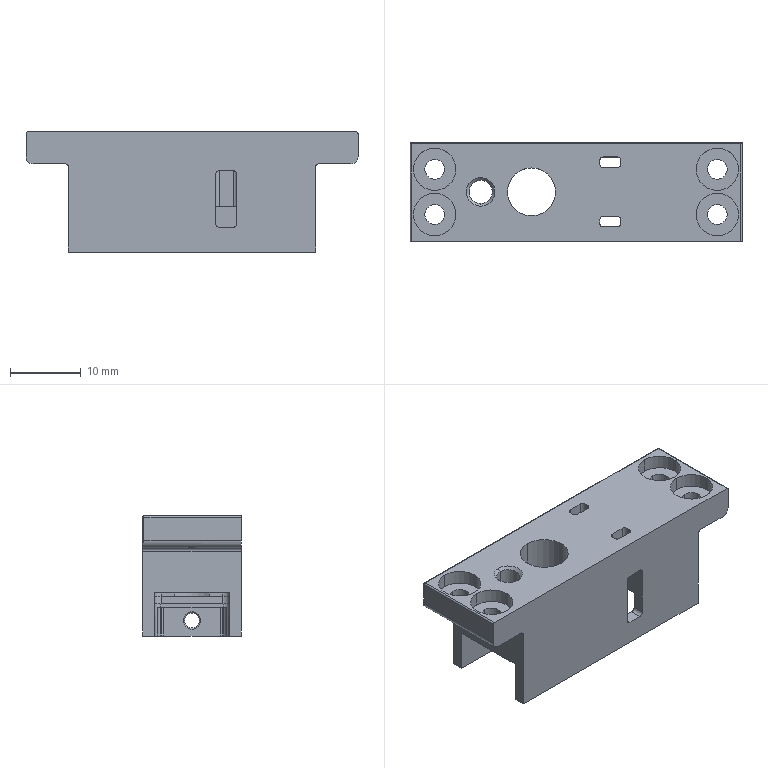NC program | NX | posted with a generic post | part box 47 x 14 x 17 mm
Lines 1496 to 2949 of 12912:
(CAVITY_MILL_COPY , TOOL : D4)
N2978 T10 M6
N2980 G54
N2982 G17 G0 G90 X8.1 Y-2.867 B0. C0. S9200 M3
N2984 G43 Z30. H10
N2986 Z0.627
N2988 G94 G1 Z-0.373 F1000.
N2990 G3 X8.887 Y-3.25 R1.
N2992 G1 X9.451 F1400.
N2994 G2 X10.016 Y-2.996 R2.
N2996 X11.2 Y-2.352 R2.14
N2998 G1 Y-1.338
N3000 G3 X10.8 Y-0.538 R1.
N3002 G1 Z0.627
N3004 G0 Z30.
N3006 X8.1 Y-2.867
N3008 Z0.255
N3010 G1 Z-0.745 F1000.
N3012 G3 X8.887 Y-3.25 R1.
N3014 G1 X9.451 F1400.
N3016 G2 X10.016 Y-2.996 R2.
N3018 X11.2 Y-2.352 R2.14
N3020 G1 Y-1.338
N3022 G3 X10.8 Y-0.538 R1.
N3024 G1 Z0.255
N3026 X8.1 Y-2.867 Z-0.118 F8000.
N3028 Z-1.118 F1000.
N3030 G3 X8.887 Y-3.25 R1.
N3032 G1 X9.451 F1400.
N3034 G2 X10.016 Y-2.996 R2.
N3036 X11.2 Y-2.352 R2.14
N3038 G1 Y-1.338
N3040 G3 X10.8 Y-0.538 R1.
N3042 G1 Z-0.118
N3044 X8.1 Y-2.867 Z-0.491 F8000.
N3046 Z-1.491 F1000.
N3048 G3 X8.887 Y-3.25 R1.
N3050 G1 X9.451 F1400.
N3052 G2 X10.016 Y-2.996 R2.
N3054 X11.2 Y-2.352 R2.14
N3056 G1 Y-1.338
N3058 G3 X10.8 Y-0.538 R1.
N3060 G1 Z-0.491
N3062 X8.1 Y-2.867 Z-0.864 F8000.
N3064 Z-1.864 F1000.
N3066 G3 X8.887 Y-3.25 R1.
N3068 G1 X9.451 F1400.
N3070 G2 X10.016 Y-2.996 R2.
N3072 X11.2 Y-2.352 R2.14
N3074 G1 Y-1.338
N3076 G3 X10.8 Y-0.538 R1.
N3078 G1 Z-0.864
N3080 X8.1 Y-2.867 Z-1.236 F8000.
N3082 Z-2.236 F1000.
N3084 G3 X8.887 Y-3.25 R1.
N3086 G1 X9.451 F1400.
N3088 G2 X10.016 Y-2.996 R2.
N3090 X11.2 Y-2.352 R2.14
N3092 G1 Y-1.338
N3094 G3 X10.8 Y-0.538 R1.
N3096 G1 Z-1.236
N3098 X8.1 Y-2.867 Z-1.609 F8000.
N3100 Z-2.609 F1000.
N3102 G3 X8.887 Y-3.25 R1.
N3104 G1 X9.451 F1400.
N3106 G2 X10.016 Y-2.996 R2.
N3108 X11.2 Y-2.352 R2.14
N3110 G1 Y-1.338
N3112 G3 X10.8 Y-0.538 R1.
N3114 G1 Z-1.609
N3116 X8.1 Y-2.867 Z-1.982 F8000.
N3118 Z-2.982 F1000.
N3120 G3 X8.887 Y-3.25 R1.
N3122 G1 X9.451 F1400.
N3124 G2 X10.016 Y-2.996 R2.
N3126 X11.2 Y-2.352 R2.14
N3128 G1 Y-1.338
N3130 G3 X10.8 Y-0.538 R1.
N3132 G1 Z-1.982
N3134 X8.1 Y-2.867 Z-2.355 F8000.
N3136 Z-3.355 F1000.
N3138 G3 X8.887 Y-3.25 R1.
N3140 G1 X9.451 F1400.
N3142 G2 X10.016 Y-2.996 R2.
N3144 X11.2 Y-2.352 R2.14
N3146 G1 Y-1.338
N3148 G3 X10.8 Y-0.538 R1.
N3150 G1 Z-2.355
N3152 X8.1 Y-2.867 Z-2.727 F8000.
N3154 Z-3.727 F1000.
N3156 G3 X8.887 Y-3.25 R1.
N3158 G1 X9.451 F1400.
N3160 G2 X10.016 Y-2.996 R2.
N3162 X11.2 Y-2.352 R2.14
N3164 G1 Y-1.338
N3166 G3 X10.8 Y-0.538 R1.
N3168 G1 Z-2.727
N3170 X8.1 Y-2.867 Z-3.1 F8000.
N3172 Z-4.1 F1000.
N3174 G3 X8.887 Y-3.25 R1.
N3176 G1 X9.451 F1400.
N3178 G2 X10.016 Y-2.996 R2.
N3180 X11.2 Y-2.352 R2.14
N3182 G1 Y-1.338
N3184 G3 X10.8 Y-0.538 R1.
N3186 G1 Z-3.1
N3188 X6.793 Y-2.95 Z-3.35 F8000.
N3190 Z-4.35 F1000.
N3192 G3 X7.593 Y-3.35 R1.
N3194 G1 X7.765 Y-3.349 F1400.
N3196 G2 X8.387 Y-3.25 R2.
N3198 G1 X8.7
N3200 Y-2.03
N3202 G3 X8.3 Y-1.23 R1.
N3204 G1 Z-3.35
N3206 X6.793 Y-2.95 Z-3.6 F8000.
N3208 Z-4.6 F1000.
N3210 G3 X7.593 Y-3.35 R1.
N3212 G1 X7.766 Y-3.349 F1400.
N3214 G2 X8.387 Y-3.25 R2.
N3216 G1 X8.7
N3218 Y-2.03
N3220 G3 X8.3 Y-1.23 R1.
N3222 G1 Z-3.6
N3224 X6.792 Y-2.95 Z-3.933 F8000.
N3226 Z-4.933 F1000.
N3228 G3 X7.592 Y-3.35 R1.
N3230 G1 X7.766 Y-3.349 F1400.
N3232 G2 X8.387 Y-3.25 R2.
N3234 G1 X8.7
N3236 Y-2.03
N3238 G3 X8.3 Y-1.23 R1.
N3240 G1 Z-3.933
N3242 X6.792 Y-2.95 Z-4.267 F8000.
N3244 Z-5.267 F1000.
N3246 G3 X7.592 Y-3.35 R1.
N3248 G1 X7.763 F1400.
N3250 X7.766 Y-3.349
N3252 G2 X8.387 Y-3.25 R2.
N3254 G1 X8.7
N3256 Y-2.03
N3258 G3 X8.3 Y-1.23 R1.
N3260 G1 Z-4.267
N3262 X6.791 Y-2.95 Z-4.6 F8000.
N3264 Z-5.6 F1000.
N3266 G3 X7.591 Y-3.35 R1.
N3268 G1 X7.763 F1400.
N3270 X7.767 Y-3.349
N3272 G2 X8.387 Y-3.25 R2.
N3274 G1 X8.7
N3276 Y-2.03
N3278 G3 X8.3 Y-1.23 R1.
N3280 G1 Z-4.6
N3282 X6.791 Y-2.95 Z-4.85 F8000.
N3284 Z-5.85 F1000.
N3286 G3 X7.591 Y-3.35 R1.
N3288 G1 X7.763 F1400.
N3290 X7.767 Y-3.349
N3292 G2 X8.387 Y-3.25 R2.
N3294 G1 X8.7
N3296 Y-2.029
N3298 G3 X8.3 Y-1.229 R1.
N3300 G1 Z-4.85
N3302 X6.791 Y-2.95 Z-5.1 F8000.
N3304 Z-6.1 F1000.
N3306 G3 X7.591 Y-3.35 R1.
N3308 G1 X7.763 F1400.
N3310 X7.767 Y-3.349
N3312 G2 X8.387 Y-3.25 R2.
N3314 G1 X8.7
N3316 Y-2.029
N3318 G3 X8.3 Y-1.229 R1.
N3320 G1 Z-5.1
N3322 X6.79 Y-2.95 Z-5.5 F8000.
N3324 Z-6.5 F1000.
N3326 G3 X7.59 Y-3.35 R1.
N3328 G1 X7.763 F1400.
N3330 X7.767 Y-3.349
N3332 G2 X8.387 Y-3.25 R2.
N3334 G1 X8.7
N3336 Y-2.029
N3338 G3 X8.3 Y-1.229 R1.
N3340 G1 Z-5.5
N3342 G0 Z30.
N3344 X10.8 Y0.538
N3346 Z0.627
N3348 G1 Z-0.373 F1000.
N3350 G3 X11.2 Y1.338 R1.
N3352 G1 Y2.352 F1400.
N3354 G2 X10.016 Y2.996 R2.14
N3356 X9.451 Y3.25 R2.
N3358 G1 X8.887
N3360 G3 X8.1 Y2.867 R1.
N3362 G1 Z0.627
N3364 G0 Z30.
N3366 X10.8 Y0.538
N3368 Z0.255
N3370 G1 Z-0.745 F1000.
N3372 G3 X11.2 Y1.338 R1.
N3374 G1 Y2.352 F1400.
N3376 G2 X10.016 Y2.996 R2.14
N3378 X9.451 Y3.25 R2.
N3380 G1 X8.887
N3382 G3 X8.1 Y2.867 R1.
N3384 G1 Z0.255
N3386 X10.8 Y0.538 Z-0.118 F8000.
N3388 Z-1.118 F1000.
N3390 G3 X11.2 Y1.338 R1.
N3392 G1 Y2.352 F1400.
N3394 G2 X10.016 Y2.996 R2.14
N3396 X9.451 Y3.25 R2.
N3398 G1 X8.887
N3400 G3 X8.1 Y2.867 R1.
N3402 G1 Z-0.118
N3404 X10.8 Y0.538 Z-0.491 F8000.
N3406 Z-1.491 F1000.
N3408 G3 X11.2 Y1.338 R1.
N3410 G1 Y2.352 F1400.
N3412 G2 X10.016 Y2.996 R2.14
N3414 X9.451 Y3.25 R2.
N3416 G1 X8.887
N3418 G3 X8.1 Y2.867 R1.
N3420 G1 Z-0.491
N3422 X10.8 Y0.538 Z-0.864 F8000.
N3424 Z-1.864 F1000.
N3426 G3 X11.2 Y1.338 R1.
N3428 G1 Y2.352 F1400.
N3430 G2 X10.016 Y2.996 R2.14
N3432 X9.451 Y3.25 R2.
N3434 G1 X8.887
N3436 G3 X8.1 Y2.867 R1.
N3438 G1 Z-0.864
N3440 X10.8 Y0.538 Z-1.236 F8000.
N3442 Z-2.236 F1000.
N3444 G3 X11.2 Y1.338 R1.
N3446 G1 Y2.352 F1400.
N3448 G2 X10.016 Y2.996 R2.14
N3450 X9.451 Y3.25 R2.
N3452 G1 X8.887
N3454 G3 X8.1 Y2.867 R1.
N3456 G1 Z-1.236
N3458 X10.8 Y0.538 Z-1.609 F8000.
N3460 Z-2.609 F1000.
N3462 G3 X11.2 Y1.338 R1.
N3464 G1 Y2.352 F1400.
N3466 G2 X10.016 Y2.996 R2.14
N3468 X9.451 Y3.25 R2.
N3470 G1 X8.887
N3472 G3 X8.1 Y2.867 R1.
N3474 G1 Z-1.609
N3476 X10.8 Y0.538 Z-1.982 F8000.
N3478 Z-2.982 F1000.
N3480 G3 X11.2 Y1.338 R1.
N3482 G1 Y2.352 F1400.
N3484 G2 X10.016 Y2.996 R2.14
N3486 X9.451 Y3.25 R2.
N3488 G1 X8.887
N3490 G3 X8.1 Y2.867 R1.
N3492 G1 Z-1.982
N3494 X10.8 Y0.538 Z-2.355 F8000.
N3496 Z-3.355 F1000.
N3498 G3 X11.2 Y1.338 R1.
N3500 G1 Y2.352 F1400.
N3502 G2 X10.016 Y2.996 R2.14
N3504 X9.451 Y3.25 R2.
N3506 G1 X8.887
N3508 G3 X8.1 Y2.867 R1.
N3510 G1 Z-2.355
N3512 X10.8 Y0.538 Z-2.727 F8000.
N3514 Z-3.727 F1000.
N3516 G3 X11.2 Y1.338 R1.
N3518 G1 Y2.352 F1400.
N3520 G2 X10.016 Y2.996 R2.14
N3522 X9.451 Y3.25 R2.
N3524 G1 X8.887
N3526 G3 X8.1 Y2.867 R1.
N3528 G1 Z-2.727
N3530 X10.8 Y0.538 Z-3.1 F8000.
N3532 Z-4.1 F1000.
N3534 G3 X11.2 Y1.338 R1.
N3536 G1 Y2.352 F1400.
N3538 G2 X10.016 Y2.996 R2.14
N3540 X9.451 Y3.25 R2.
N3542 G1 X8.887
N3544 G3 X8.1 Y2.867 R1.
N3546 G1 Z-3.1
N3548 X8.3 Y1.231 Z-3.35 F8000.
N3550 Z-4.35 F1000.
N3552 G3 X8.7 Y2.031 R1.
N3554 G1 Y3.25 F1400.
N3556 X8.387
N3558 G2 X7.763 Y3.35 R2.
N3560 G1 X7.596
N3562 G3 X6.796 Y2.95 R1.
N3564 G1 Z-3.35
N3566 X8.3 Y1.231 Z-3.6 F8000.
N3568 Z-4.6 F1000.
N3570 G3 X8.7 Y2.031 R1.
N3572 G1 Y3.25 F1400.
N3574 X8.387
N3576 G2 X7.763 Y3.35 R2.
N3578 G1 X7.596
N3580 G3 X6.796 Y2.95 R1.
N3582 G1 Z-3.6
N3584 X8.3 Y1.231 Z-3.933 F8000.
N3586 Z-4.933 F1000.
N3588 G3 X8.7 Y2.031 R1.
N3590 G1 Y3.25 F1400.
N3592 X8.387
N3594 G2 X7.763 Y3.35 R2.
N3596 G1 X7.596
N3598 G3 X6.796 Y2.95 R1.
N3600 G1 Z-3.933
N3602 X8.3 Y1.231 Z-4.267 F8000.
N3604 Z-5.267 F1000.
N3606 G3 X8.7 Y2.031 R1.
N3608 G1 Y3.25 F1400.
N3610 X8.387
N3612 G2 X7.763 Y3.35 R2.
N3614 G1 X7.596
N3616 G3 X6.796 Y2.95 R1.
N3618 G1 Z-4.267
N3620 X8.3 Y1.231 Z-4.6 F8000.
N3622 Z-5.6 F1000.
N3624 G3 X8.7 Y2.031 R1.
N3626 G1 Y3.25 F1400.
N3628 X8.387
N3630 G2 X7.763 Y3.35 R2.
N3632 G1 X7.596
N3634 G3 X6.796 Y2.95 R1.
N3636 G1 Z-4.6
N3638 X8.3 Y1.231 Z-4.85 F8000.
N3640 Z-5.85 F1000.
N3642 G3 X8.7 Y2.031 R1.
N3644 G1 Y3.25 F1400.
N3646 X8.387
N3648 G2 X7.763 Y3.35 R2.
N3650 G1 X7.596
N3652 G3 X6.796 Y2.95 R1.
N3654 G1 Z-4.85
N3656 X8.3 Y1.231 Z-5.1 F8000.
N3658 Z-6.1 F1000.
N3660 G3 X8.7 Y2.031 R1.
N3662 G1 Y3.25 F1400.
N3664 X8.387
N3666 G2 X7.763 Y3.35 R2.
N3668 G1 X7.596
N3670 G3 X6.796 Y2.95 R1.
N3672 G1 Z-5.1
N3674 X8.3 Y1.231 Z-5.5 F8000.
N3676 Z-6.5 F1000.
N3678 G3 X8.7 Y2.031 R1.
N3680 G1 Y3.25 F1400.
N3682 X8.387
N3684 G2 X7.763 Y3.35 R2.
N3686 G1 X7.596
N3688 G3 X6.796 Y2.95 R1.
N3690 G1 Z-5.5
N3692 G0 Z30.
N3694 X3.699
N3696 Z-3.933
N3698 G1 Z-4.933 F1000.
N3700 G3 X2.899 Y3.35 R1.
N3702 G1 X1.6 F1400.
N3704 Y2.051
N3706 G3 X2. Y1.251 R1.
N3708 G1 Z-3.933
N3710 X3.699 Y2.95 Z-4.267 F8000.
N3712 Z-5.267 F1000.
N3714 G3 X2.899 Y3.35 R1.
N3716 G1 X1.6 F1400.
N3718 Y2.051
N3720 G3 X2. Y1.251 R1.
N3722 G1 Z-4.267
N3724 X3.699 Y2.95 Z-4.6 F8000.
N3726 Z-5.6 F1000.
N3728 G3 X2.899 Y3.35 R1.
N3730 G1 X1.6 F1400.
N3732 Y2.051
N3734 G3 X2. Y1.251 R1.
N3736 G1 Z-4.6
N3738 X3.699 Y2.95 Z-4.85 F8000.
N3740 Z-5.85 F1000.
N3742 G3 X2.899 Y3.35 R1.
N3744 G1 X1.6 F1400.
N3746 Y2.051
N3748 G3 X2. Y1.251 R1.
N3750 G1 Z-4.85
N3752 X3.699 Y2.95 Z-5.1 F8000.
N3754 Z-6.1 F1000.
N3756 G3 X2.899 Y3.35 R1.
N3758 G1 X1.6 F1400.
N3760 Y2.051
N3762 G3 X2. Y1.251 R1.
N3764 G1 Z-5.1
N3766 X3.699 Y2.95 Z-5.5 F8000.
N3768 Z-6.5 F1000.
N3770 G3 X2.899 Y3.35 R1.
N3772 G1 X1.6 F1400.
N3774 Y2.051
N3776 G3 X2. Y1.251 R1.
N3778 G1 Z-5.5
N3780 G0 Z30.
N3782 Y-1.251
N3784 Z-3.933
N3786 G1 Z-4.933 F1000.
N3788 G3 X1.6 Y-2.051 R1.
N3790 G1 Y-3.35 F1400.
N3792 X2.899
N3794 G3 X3.699 Y-2.95 R1.
N3796 G1 Z-3.933
N3798 X2. Y-1.251 Z-4.267 F8000.
N3800 Z-5.267 F1000.
N3802 G3 X1.6 Y-2.051 R1.
N3804 G1 Y-3.35 F1400.
N3806 X2.899
N3808 G3 X3.699 Y-2.95 R1.
N3810 G1 Z-4.267
N3812 X2. Y-1.251 Z-4.6 F8000.
N3814 Z-5.6 F1000.
N3816 G3 X1.6 Y-2.051 R1.
N3818 G1 Y-3.35 F1400.
N3820 X2.899
N3822 G3 X3.699 Y-2.95 R1.
N3824 G1 Z-4.6
N3826 X2. Y-1.251 Z-4.85 F8000.
N3828 Z-5.85 F1000.
N3830 G3 X1.6 Y-2.051 R1.
N3832 G1 Y-3.35 F1400.
N3834 X2.899
N3836 G3 X3.699 Y-2.95 R1.
N3838 G1 Z-4.85
N3840 X2. Y-1.251 Z-5.1 F8000.
N3842 Z-6.1 F1000.
N3844 G3 X1.6 Y-2.051 R1.
N3846 G1 Y-3.35 F1400.
N3848 X2.899
N3850 G3 X3.699 Y-2.95 R1.
N3852 G1 Z-5.1
N3854 X2. Y-1.251 Z-5.5 F8000.
N3856 Z-6.5 F1000.
N3858 G3 X1.6 Y-2.051 R1.
N3860 G1 Y-3.35 F1400.
N3862 X2.899
N3864 G3 X3.699 Y-2.95 R1.
N3866 G1 Z-5.5
N3868 G0 Z30.
N3870 X-6.099
N3872 Z-3.933
N3874 G1 Z-4.933 F1000.
N3876 G3 X-5.299 Y-3.35 R1.
N3878 G1 X-4. F1400.
N3880 Y-2.051
N3882 G3 X-4.4 Y-1.251 R1.
N3884 G1 Z-3.933
N3886 X-6.099 Y-2.95 Z-4.267 F8000.
N3888 Z-5.267 F1000.
N3890 G3 X-5.299 Y-3.35 R1.
N3892 G1 X-4. F1400.
N3894 Y-2.051
N3896 G3 X-4.4 Y-1.251 R1.
N3898 G1 Z-4.267
N3900 X-6.099 Y-2.95 Z-4.6 F8000.
N3902 Z-5.6 F1000.
N3904 G3 X-5.299 Y-3.35 R1.
N3906 G1 X-4. F1400.
N3908 Y-2.051
N3910 G3 X-4.4 Y-1.251 R1.
N3912 G1 Z-4.6
N3914 X-7.098 Y-2.95 Z-4.85 F8000.
N3916 Z-5.85 F1000.
N3918 G3 X-6.298 Y-3.35 R1.
N3920 G1 X-5. F1400.
N3922 Y-2.433
N3924 G2 X-4.964 Y-2.058 R2.
N3926 G3 X-5.12 Y-1.308 R1.
N3928 G1 Z-4.85
N3930 X-7.098 Y-2.95 Z-5.1 F8000.
N3932 Z-6.1 F1000.
N3934 G3 X-6.298 Y-3.35 R1.
N3936 G1 X-5. F1400.
N3938 Y-2.433
N3940 G2 X-4.964 Y-2.058 R2.
N3942 G3 X-5.12 Y-1.308 R1.
N3944 G1 Z-5.1
N3946 G0 Z30.
N3948 X-4.4 Y1.251
N3950 Z-3.933
N3952 G1 Z-4.933 F1000.
N3954 G3 X-4. Y2.051 R1.
N3956 G1 Y3.35 F1400.
N3958 X-5.299
N3960 G3 X-6.099 Y2.95 R1.
N3962 G1 Z-3.933
N3964 X-4.4 Y1.251 Z-4.267 F8000.
N3966 Z-5.267 F1000.
N3968 G3 X-4. Y2.051 R1.
N3970 G1 Y3.35 F1400.
N3972 X-5.299
N3974 G3 X-6.099 Y2.95 R1.
N3976 G1 Z-4.267
N3978 X-4.4 Y1.251 Z-4.6 F8000.
N3980 Z-5.6 F1000.
N3982 G3 X-4. Y2.051 R1.
N3984 G1 Y3.35 F1400.
N3986 X-5.299
N3988 G3 X-6.099 Y2.95 R1.
N3990 G1 Z-4.6
N3992 X-5.12 Y1.308 Z-4.85 F8000.
N3994 Z-5.85 F1000.
N3996 G3 X-4.964 Y2.058 R1.
N3998 G2 X-5. Y2.433 R2. F1400.
N4000 G1 Y3.35
N4002 X-6.298
N4004 G3 X-7.098 Y2.95 R1.
N4006 G1 Z-4.85
N4008 X-5.12 Y1.308 Z-5.1 F8000.
N4010 Z-6.1 F1000.
N4012 G3 X-4.964 Y2.058 R1.
N4014 G2 X-5. Y2.433 R2. F1400.
N4016 G1 Y3.35
N4018 X-6.298
N4020 G3 X-7.098 Y2.95 R1.
N4022 G1 Z-5.1
N4024 G0 Z30.
(FLOOR_WALL_COPY_COPY , TOOL : D4)
N4026 X25.808 Y9.734 S9500
N4028 Z-11.
N4030 G1 Z-12.5 F1000.
N4032 X24.996 Y9.591
N4034 G3 X24.5 Y9. R0.6
N4036 G1 Y-9.
N4038 X20.2
N4040 Y9.
N4042 X24.5
N4044 X22.7 Y7.2
N4046 Y-7.2
N4048 X22.
N4050 Y7.2
N4052 X22.7
N4054 G3 X23.291 Y7.696 R0.6
N4056 G1 X23.785 Y10.5
N4058 Z-11.
N4060 G0 Z30.
N4062 X20.496
N4064 Z-11.
N4066 G1 Z-12.5
N4068 Y9.591
N4070 G3 X20. Y9. R0.6
N4072 G1 Y-9.
N4074 G3 X20.496 Y-9.591 R0.6
N4076 G1 Y-10.5
N4078 Z-11.
N4080 G0 Z30.
N4082 X7.2 Y-1.85
N4084 Z-2.6
N4086 G1 Z-4.1
N4088 X9.196 Y-2.459
N4090 G3 X8.7 Y-3.05 R0.6
N4092 G1 Y3.05
N4094 X9.393
N4096 G3 X9.909 Y2.818 R2.2
N4098 X11. Y2.191 R2.34
N4100 G1 Y-2.191
N4102 G3 X9.909 Y-2.818 R2.34
N4104 X9.393 Y-3.05 R2.2
N4106 G1 X8.7
N4108 G3 X9.291 Y-2.554 R0.6
N4110 G1 X7.2 Y-1.85
N4112 Z-2.6
N4114 G0 Z30.
N4116 Z-2.6
N4118 G1 Z-4.1
N4120 X8.109 Y-2.754
N4122 G3 X8.7 Y-3.25 R0.6
N4124 G1 X9.451
N4126 G2 X10.016 Y-2.996 R2.
N4128 X11.2 Y-2.352 R2.14
N4130 G1 Y2.352
N4132 G2 X10.016 Y2.996 R2.14
N4134 X9.451 Y3.25 R2.
N4136 G1 X8.7
N4138 G3 X8.109 Y2.754 R0.6
N4140 G1 X7.2 Y1.85
N4142 Z-2.6
N4144 G0 Z30.
N4146 X7.141 Y-2.654
N4148 Z-5.
N4150 G1 Z-6.5
N4152 G3 X7.732 Y-3.15 R0.6
N4154 G1 X1.8
N4156 Y3.15
N4158 X7.732
N4160 G3 X8.387 Y3.05 R2.2
N4162 G1 X8.5
N4164 Y-3.05
N4166 X8.387
N4168 G3 X7.732 Y-3.15 R2.2
N4170 G1 X6.1 Y-0.75
N4172 X4.2
N4174 Y0.75
N4176 X6.1
N4178 Y-0.75
N4180 X8.204 Y-1.341
N4182 G3 X8.7 Y-0.75 R0.6
N4184 G1 Y3.25
N4186 X8.387
N4188 G2 X7.763 Y3.35 R2.
N4190 G1 X1.6
N4192 Y-3.35
N4194 X7.763
N4196 G2 X8.387 Y-3.25 R2.
N4198 G1 X8.7
N4200 Y-0.75
N4202 G3 X8.204 Y-0.159 R0.6
N4204 G1 X7.2 Y0.018
N4206 Z-5.
N4208 G0 Z30.
N4210 X3.1 Y1.85
N4212 Z-3.1
N4214 G1 Z-4.6
N4216 X1.104 Y2.559
N4218 G3 X1.6 Y3.15 R0.6
N4220 G1 Y-3.15
N4222 X-4.
N4224 Y3.15
N4226 X1.6
N4228 X-0.8 Y0.75
N4230 Y-0.75
N4232 X-1.6
N4234 Y0.75
N4236 X-0.8
N4238 G3 X-0.209 Y1.246 R0.6
N4240 G1 X3.1
N4242 Z-3.1
N4244 G0 Z30.
N4246 Y1.85
N4248 Z-3.1
N4250 G1 Z-4.6
N4252 X2.191 Y2.854
N4254 G3 X1.6 Y3.35 R0.6
N4256 G1 X-4.
N4258 G3 X-4.591 Y2.854 R0.6
N4260 G1 X-5.5 Y1.85
N4262 Z-3.1
N4264 G0 Z30.
N4266 Y-1.85
N4268 Z-3.1
N4270 G1 Z-4.6
N4272 X-4.591 Y-2.854
N4274 G3 X-4. Y-3.35 R0.6
N4276 G1 X1.59
N4278 G3 X2.181 Y-2.854 R0.6
N4280 G1 X3.1 Y-1.85
N4282 Z-3.1
N4284 G0 Z30.
N4286 X-5.733
N4288 Z-4.1
N4290 G1 Z-5.6
N4292 X-5.591 Y-2.654
N4294 G3 X-5. Y-3.15 R0.6
N4296 G1 X-4.2
N4298 Y3.15
N4300 X-5.
N4302 G3 X-5.615 Y2.685 R0.6
N4304 G1 X-5.806 Y1.85
N4306 Z-4.1
N4308 G0 Z30.
N4310 X-5.99 Y-0.591
N4312 Z-4.1
N4314 G1 Z-5.6
N4316 X-5.591 Y-2.854
N4318 G3 X-5. Y-3.35 R0.6
N4320 G1 X-4.
N4322 Y3.35
N4324 X-4.99
N4326 G3 X-5.581 Y2.854 R0.6
N4328 G1 X-5.982 Y0.58
N4330 Z-4.1
N4332 G0 Z30.
N4334 X-6.052 Y0.546
N4336 Z-4.6
N4338 G1 Z-6.1
N4340 X-5.322 Y2.155
N4342 G3 X-5.2 Y1.789 R0.3
N4344 X-5.2 Y-1.789 R-2.1
N4346 G1 Y-3.15
N4348 X-19.5
N4350 Y3.15
N4352 X-5.2
N4354 Y1.789
N4356 G3 X-7.974 Y1.268 R2.1
N4358 G1 X-10.737 Y0.75
N4360 G3 X-10.737 Y-0.75 R4.5
N4362 G1 X-17.1
N4364 Y0.75
N4366 X-10.737
N4368 G3 X-10.146 Y1.246 R0.6
N4370 G1 X-6.871 Y0.185
N4372 Z-4.6
N4374 G0 Z30.
N4376 X-5.747 Y0.233
N4378 Z-4.6
N4380 G1 Z-6.1
N4382 X-4.78 Y0.642
N4384 G3 X-4.732 Y1.411 R0.6
N4386 G1 X-5. Y1.776
N4388 Y3.35
N4390 X-19.5
N4392 G3 X-20.091 Y2.854 R0.6
N4394 G1 X-21.
N4396 Z-4.6
N4398 G0 Z30.
N4400 Y-2.854
N4402 Z-4.6
N4404 G1 Z-6.1
N4406 X-20.091
N4408 G3 X-19.5 Y-3.35 R0.6
N4410 G1 X-5.
N4412 Y-1.776
N4414 X-4.732 Y-1.411
N4416 G3 X-4.78 Y-0.642 R0.6
N4418 G1 X-5.747 Y-0.233
N4420 Z-4.6
N4422 G0 Z30.
N4424 X-25.808 Y-9.734
N4426 Z-11.
N4428 G1 Z-12.5
N4430 X-24.996 Y-9.591
N4432 G3 X-24.5 Y-9. R0.6
N4434 G1 Y9.
N4436 X-20.2
N4438 Y-9.
N4440 X-24.5
N4442 X-22.7 Y-7.2
N4444 Y7.2
N4446 X-22.
N4448 Y-7.2
N4450 X-22.7
N4452 G3 X-23.291 Y-7.696 R0.6
N4454 G1 X-23.785 Y-10.5
N4456 Z-11.
N4458 G0 Z30.
N4460 X-20.496
N4462 Z-11.
N4464 G1 Z-12.5
N4466 Y-9.591
N4468 G3 X-20. Y-9. R0.6
N4470 G1 Y9.
N4472 G3 X-20.496 Y9.591 R0.6
N4474 G1 Y10.5
N4476 Z-11.
N4478 G0 Z30.
(ZLEVEL_PROFILE_COPY_COPY , TOOL : D4)
N4480 X20.225 Y9.83 S8000
N4482 Z-6.
N4484 G1 X19.697 Y9.524 F1200.
N4486 G3 X19.497 Y9.177 R0.4
N4488 G1 X19.5 Y6.636
N4490 Y-7.
N4492 X19.498 Y-7.306
N4494 X19.499 Y-8.895
N4496 X19.497 Y-9.177
N4498 G3 X19.694 Y-9.525 R0.4
N4500 G1 X20.224 Y-9.837
N4502 G0 X20.226 Y9.83 Z-12.
N4504 G1 X19.697 Y9.524
N4506 G3 X19.498 Y9.177 R0.4
N4508 G1 X19.5 Y6.636
N4510 Y-7.
N4512 Y-8.895
N4514 X19.498 Y-9.177
N4516 G3 X19.695 Y-9.525 R0.4
N4518 G1 X20.225 Y-9.837
N4520 G0 Z30.
N4522 X-20.227 Y-9.83
N4524 Z-6.
N4526 G1 X-19.698 Y-9.524
N4528 G3 X-19.498 Y-9.177 R0.4
N4530 G1 X-19.5 Y-6.99
N4532 Y5.542
N4534 X-19.501 Y8.895
N4536 X-19.498 Y9.177
N4538 G3 X-19.695 Y9.526 R0.4
N4540 G1 X-20.225 Y9.838
N4542 G0 X-20.228 Y-9.829 Z-12.
N4544 G1 X-19.699 Y-9.524
N4546 G3 X-19.499 Y-9.177 R0.4
N4548 G1 X-19.5 Y-6.99
N4550 Y5.524
N4552 X-19.499 Y9.177
N4554 G3 X-19.699 Y9.524 R0.4
N4556 G1 X-20.228 Y9.829
N4558 G0 Z30.
(ZLEVEL_PROFILE_COPY_COPY_COPY , TOOL : D4)
N4560 X20.242 Y9.839
N4562 Z-12.05
N4564 G1 X19.717 Y9.535 F2500.
N4566 G3 X19.517 Y9.188 R0.4
N4568 G1 X19.518 Y8.048
N4570 X19.514 Y7.765
N4572 G2 X19.502 Y7. R10.147
N4574 G1 Y-7.
N4576 G2 X19.519 Y-9.189 R107.631
N4578 G1 X19.53 Y-9.19 Z-12.074
N4580 X19.538 Z-12.099
N4582 G3 X19.51 Y-7. R53.311
N4584 G1 Y7.
N4586 G3 X19.526 Y7.765 R6.555
N4588 G1 X19.536 Y8.048
N4590 X19.535 Y9.19
N4592 X19.548 Z-12.123
N4594 X19.556 Y9.191 Z-12.147
N4596 G2 X19.536 Y7.271 R40.111
N4598 X19.522 Y7. R8.794
N4600 G1 Y-7.
N4602 G2 X19.56 Y-9.191 R36.167
N4604 G1 X19.575 Y-9.193 Z-12.17
N4606 X19.587 Z-12.193
N4608 G3 X19.539 Y-7. R38.244
N4610 G1 Y7.
N4612 G3 X19.583 Y9.193 R27.926
N4614 G1 X19.613 Y9.194 Z-12.237
N4616 G2 X19.56 Y6.851 R36.187
N4618 G1 Y-6.869
N4620 G2 X19.616 Y-9.195 R35.374
N4622 G1 X19.629 Y-9.196 Z-12.257
N4624 X19.646 Y-9.197 Z-12.278
N4626 G3 X19.584 Y-6.833 R31.964
N4628 G1 Y6.833
N4630 G3 X19.644 Y9.196 R26.898
N4632 G1 X19.654 Y9.197 Z-12.297
N4634 X19.672 Y9.199 Z-12.315
N4636 G2 X19.612 Y6.867 R25.484
N4638 G1 Y-6.867
N4640 G2 X19.673 Y-9.199 R26.442
N4642 G1 X19.693 Z-12.332
N4644 X19.707 Y-9.2 Z-12.349
N4646 G3 X19.642 Y-7. R19.819
N4648 G1 Y7.
N4650 G3 X19.709 Y9.198 R20.233
N4652 G1 X19.754 Y9.193 Z-12.379
N4654 G2 X19.673 Y6.883 R21.682
N4656 G1 X19.68 Y-6.883
N4658 G2 X19.75 Y-9.199 R22.706
N4660 G1 X19.786 Z-12.404
N4662 G3 X19.705 Y-6.833 R19.562
N4664 G1 Y6.833
N4666 G3 X19.792 Y9.189 R22.773
N4668 G1 X19.823 Y9.186 Z-12.424
N4670 G2 X19.735 Y6.831 R22.854
N4672 G1 Y-6.831
N4674 G2 X19.815 Y-9.198 R19.694
N4676 G1 X19.849 Z-12.441
N4678 G3 X19.765 Y-6.865 R17.61
N4680 G1 Y6.865
N4682 G3 X19.86 Y9.184 R34.945
N4684 G1 X19.87 Z-12.448
N4686 X19.892 Y9.183 Z-12.456
N4688 G2 X19.794 Y7. R16.388
N4690 G1 Y-6.99
N4692 G2 X19.873 Y-7.765 R5.774
N4694 G1 X19.884 Y-8.048
N4696 X19.883 Y-9.198
N4698 X19.89 Y-9.199 Z-12.461
N4700 X19.911 Z-12.467
N4702 Y-8.048
N4704 X19.9 Y-7.563
N4706 G3 X19.822 Y-6.985 R2.641
N4708 G1 Y7.
N4710 G3 X19.918 Y9.181 R17.105
N4712 G1 X19.917 Z-12.471
N4714 X19.937 Z-12.475
N4716 X19.928 Y8.048
N4718 X19.912 Y7.765
N4720 X19.845 Y7.
N4722 Y-6.97
N4724 G2 X19.926 Y-7.623 R2.727
N4726 G1 X19.931 Y-9.199
N4728 X19.93 Z-12.478
N4730 X19.945 Z-12.481
N4732 X19.943 Y-7.626
N4734 G3 X19.864 Y-6.966 R2.875
N4736 G1 Y7.
N4738 G3 X19.943 Y8.33 R11.571
N4740 G1 X19.95 Y9.18
N4742 X19.959 Y9.179 Z-12.485
N4744 X19.952 Y8.33
N4746 G2 X19.88 Y7. R12.686
N4748 G1 Y-6.993
N4750 G2 X19.953 Y-7.574 R2.338
N4752 G1 X19.955 Y-9.2
N4754 X19.965 Z-12.489
N4756 X19.967 Y-7.483
N4758 X19.965 Y-7.406
N4760 X19.924 Y-6.995
N4762 X19.897 Y-6.99
N4764 Y6.921
N4766 G3 X19.969 Y9.179 R24.593
N4768 G1 X20.003 Y9.16 Z-12.5
N4770 X20.005 Y9.142
N4772 X19.965 Y6.809
N4774 X19.95 Y6.636
N4776 X19.984 Y-6.918
N4778 X20.002 Y-9.16
N4780 G3 X20.205 Y-9.504 R0.4
N4782 G1 X20.733 Y-9.804
N4784 G0 Z30.
N4786 X-20.243 Y-9.839
N4788 Z-12.05
N4790 G1 X-19.717 Y-9.535
N4792 G3 X-19.517 Y-9.189 R0.4
N4794 G1 X-19.518 Y-8.048
N4796 X-19.514 Y-7.765
N4798 G2 X-19.502 Y-7. R10.125
N4800 G1 Y7.
N4802 X-19.507 Y7.201
N4804 X-19.519 Y9.189
N4806 X-19.53 Z-12.074
N4808 X-19.538 Y9.19 Z-12.099
N4810 G3 X-19.51 Y7. R54.461
N4812 G1 Y-7.
N4814 G3 X-19.526 Y-7.765 R6.56
N4816 G1 X-19.536 Y-8.048
N4818 X-19.535 Y-9.19
N4820 X-19.548 Y-9.191 Z-12.123
N4822 X-19.556 Z-12.147
N4824 G2 X-19.536 Y-7.273 R40.252
N4826 X-19.522 Y-7. R8.65
N4828 G1 Y7.
N4830 G2 X-19.56 Y9.191 R36.165
N4832 G1 X-19.575 Y9.192 Z-12.17
N4834 X-19.587 Y9.193 Z-12.193
N4836 G3 X-19.539 Y7. R38.242
N4838 G1 Y-7.
N4840 G3 X-19.583 Y-9.193 R28.064
N4842 G1 X-19.613 Y-9.195 Z-12.237
N4844 G2 X-19.56 Y-6.869 R28.279
N4846 G1 Y6.851
N4848 G2 X-19.616 Y9.195 R35.64
N4850 G1 X-19.629 Z-12.257
N4852 X-19.646 Y9.196 Z-12.278
N4854 G3 X-19.584 Y6.833 R31.962
N4856 G1 Y-6.833
N4858 G3 X-19.644 Y-9.196 R26.891
N4860 G1 X-19.654 Y-9.197 Z-12.297
N4862 X-19.672 Y-9.199 Z-12.315
N4864 G2 X-19.612 Y-6.867 R25.503
N4866 G1 Y6.867
N4868 G2 X-19.673 Y9.199 R26.465
N4870 G1 X-19.693 Z-12.332
N4872 X-19.707 Z-12.349
N4874 G3 X-19.642 Y7. R19.506
N4876 G1 Y-7.
N4878 G3 X-19.709 Y-9.198 R20.233
N4880 G1 X-19.754 Y-9.193 Z-12.379
N4882 G2 X-19.673 Y-6.883 R21.686
N4884 G1 Y6.883
N4886 G2 X-19.75 Y9.199 R19.878
N4888 G1 X-19.786 Z-12.404
N4890 G3 X-19.705 Y6.828 R19.699
N4892 G1 Y-6.833
N4894 G3 X-19.792 Y-9.19 R22.689
N4896 G1 X-19.823 Y-9.187 Z-12.424
N4898 G2 X-19.735 Y-6.831 R22.852
N4900 G1 Y6.824
N4902 G2 X-19.815 Y9.198 R19.895
N4904 G1 X-19.849 Z-12.441
N4906 G3 X-19.765 Y6.864 R17.785
N4908 G1 Y-6.865
N4910 G3 X-19.86 Y-9.184 R22.052
N4912 G1 X-19.87 Z-12.448
N4914 X-19.892 Y-9.183 Z-12.456
N4916 G2 X-19.794 Y-7. R16.368
N4918 G1 Y6.984
N4920 X-19.814 Y7.012
N4922 X-19.884 Y8.048
N4924 X-19.883 Y9.198
N4926 X-19.89 Y9.199 Z-12.461
N4928 X-19.911 Z-12.467
N4930 Y8.048
N4932 G3 X-19.822 Y6.99 R5.202
N4934 G1 Y-7.
N4936 G3 X-19.918 Y-9.182 R17.103
N4938 G1 X-19.917 Z-12.471
N4940 X-19.937 Y-9.181 Z-12.475
N4942 G2 X-19.868 Y-7.063 R25.579
N4944 G1 X-19.845 Y-7.
N4946 Y6.966
N4948 X-19.894 Y7.238
N4950 X-19.883 Y7.301
N4952 X-19.916 Y7.326
N4954 X-19.917 Y7.367
N4956 X-19.927 Y7.765
N4958 X-19.931 Y9.199
N4960 X-19.93 Z-12.478
N4962 X-19.945 Z-12.481
N4964 X-19.939 Y7.483
N4966 G3 X-19.864 Y6.974 R8.803
N4968 G1 Y-7.
N4970 X-19.884 Y-7.061
N4972 X-19.942 Y-8.048
N4974 X-19.95 Y-9.18
N4976 X-19.959 Z-12.485
N4978 X-19.952 Y-8.33
N4980 G2 X-19.88 Y-7. R12.63
N4982 G1 Y6.992
N4984 G2 X-19.954 Y7.586 R2.439
N4986 G1 X-19.955 Y9.2
N4988 X-19.966 Y9.194 Z-12.489
N4990 X-19.967 Y7.483
N4992 X-19.965 Y7.332
N4994 X-19.924 Y6.996
N4996 X-19.897 Y6.99
N4998 Y-7.
N5000 G3 X-19.969 Y-9.194 R21.708
N5002 G1 X-19.984 Y-9.078 Z-12.495
N5004 X-20.002 Y-8.962 Z-12.5
N5006 X-19.965 Y-6.809
N5008 X-19.95 Y-6.636
N5010 Y6.636
N5012 X-19.993 Y6.918
N5014 X-20.002 Y9.034
N5016 G3 X-20.203 Y9.38 R0.4
N5018 G1 X-20.755 Y9.695
N5020 G0 Z30.
(ZLEVEL_PROFILE_COPY_COPY_COPY_COPY , TOOL : D4)
N5022 X25.26 Y9.812
N5024 Z-12.506
N5026 G1 X24.739 Y9.541
N5028 G3 X24.524 Y9.203 R0.4
N5030 X24.612 Y7. R13.237
N5032 G1 Y-7.
N5034 X24.585 Y-7.201
N5036 X24.524 Y-8.895
N5038 X24.519 Y-9.204
N5040 X24.556 Y-9.2 Z-12.513
N5042 G2 X24.66 Y-7. R17.792
N5044 G1 Y7.
N5046 X24.563 Y7.765
N5048 X24.562 Y9.2
N5050 X24.583 Z-12.517
N5052 X24.59 Z-12.52
N5054 G3 X24.7 Y7. R11.703
N5056 G1 Y-7.
N5058 G3 X24.581 Y-9.2 R17.927
N5060 G1 X24.606 Z-12.524
N5062 X24.61 Z-12.528
N5064 G2 X24.736 Y-7. R19.59
N5066 G1 Y7.
N5068 G2 X24.621 Y9.201 R11.617
N5070 G1 X24.648 Z-12.533
N5072 X24.656 Z-12.537
N5074 G3 X24.771 Y7. R12.161
N5076 G1 Y-7.
N5078 G3 X24.642 Y-9.201 R19.992
N5080 G1 X24.666 Z-12.542
N5082 X24.676 Z-12.547
N5084 G2 X24.803 Y-7. R19.155
N5086 G1 Y7.
N5088 G2 X24.694 Y9.202 R12.218
N5090 G1 X24.713 Y9.201 Z-12.553
N5092 X24.722 Z-12.558
N5094 G3 X24.836 Y7. R11.959
N5096 G1 Y-7.
N5098 G3 X24.71 Y-9.201 R16.841
N5100 G1 X24.731 Z-12.565
N5102 X24.743 Z-12.571
N5104 G2 X24.87 Y-7. R16.368
N5106 G1 Y7.
N5108 G2 X24.755 Y9.201 R12.655
N5110 G1 X24.78 Y9.2 Z-12.579
N5112 X24.792 Z-12.586
N5114 G3 X24.906 Y7. R12.775
N5116 G1 Y-7.
N5118 G3 X24.78 Y-9.2 R16.674
N5120 G1 X24.805 Z-12.594
N5122 X24.823 Z-12.603
N5124 G2 X24.942 Y-7. R17.417
N5126 G1 Y7.
N5128 G2 X24.833 Y9.2 R13.717
N5130 G1 X24.875 Z-12.622
N5132 G3 X24.978 Y7. R15.466
N5134 G1 Y-7.
N5136 G3 X24.868 Y-9.2 R18.616
N5138 G1 X24.919 Y-9.202 Z-12.643
N5140 G2 X25.016 Y-7. R21.512
N5142 G1 Y7.
N5144 G2 X24.922 Y9.201 R18.845
N5146 G1 X24.975 Y9.203 Z-12.667
N5148 G3 X25.054 Y7. R19.712
N5150 G1 Y-7.
N5152 G3 X24.975 Y-9.203 R19.858
N5154 G1 X24.991 Z-12.681
N5156 X25.011 Y-9.202 Z-12.694
N5158 G2 X25.092 Y-7. R18.54
N5160 G1 Y7.
N5162 G2 X25.011 Y9.201 R18.5
N5164 G1 X25.031 Z-12.708
N5166 X25.048 Z-12.722
N5168 G3 X25.128 Y7. R18.918
N5170 G1 Y-7.
N5172 G3 X25.048 Y-9.201 R18.944
N5174 G1 X25.07 Z-12.737
N5176 X25.088 Y-9.2 Z-12.753
N5178 G2 X25.164 Y-7. R20.198
N5180 G1 Y7.
N5182 G2 X25.088 Y9.2 R20.192
N5184 G1 X25.111 Z-12.769
N5186 X25.129 Z-12.785
N5188 G3 X25.199 Y7. R22.79
N5190 G1 Y-7.
N5192 G3 X25.129 Y-9.2 R22.795
N5194 G1 X25.154 Y-9.201 Z-12.802
N5196 X25.169 Z-12.819
N5198 G2 X25.233 Y-7. R26.734
N5200 G1 Y7.
N5202 G2 X25.169 Y9.201 R26.729
N5204 G1 X25.204 Y9.202 Z-12.856
N5206 G3 X25.265 Y7. R25.249
N5208 G1 Y-7.
N5210 G3 X25.204 Y-9.202 R25.251
N5212 G1 X25.22 Z-12.875
N5214 X25.233 Z-12.894
N5216 G2 X25.295 Y-7. R24.181
N5218 G1 Y7.
N5220 G2 X25.233 Y9.202 R24.181
N5222 G1 X25.25 Z-12.914
N5224 X25.263 Z-12.933
N5226 G3 X25.324 Y7. R25.164
N5228 G1 Y-7.
N5230 G3 X25.263 Y-9.202 R25.162
N5232 G1 X25.281 Z-12.954
N5234 X25.295 Z-12.974
N5236 G2 X25.351 Y-7. R27.207
N5238 G1 Y7.
N5240 G2 X25.295 Y9.202 R27.211
N5242 G1 X25.309 Z-12.996
N5244 X25.327 Y9.203 Z-13.017
N5246 G3 X25.376 Y7. R31.039
N5248 G1 Y-7.
N5250 G3 X25.327 Y-9.203 R30.482
N5252 G1 X25.335 Y-9.202 Z-13.039
N5254 X25.348 Z-13.061
N5256 G2 X25.399 Y-7. R27.979
N5258 G1 Y7.
N5260 G2 X25.347 Y9.202 R30.707
N5262 G1 X25.366 Y9.201 Z-13.106
N5264 G3 X25.419 Y7. R32.882
N5266 G1 Y-7.
N5268 G3 X25.369 Y-9.201 R28.457
N5270 G1 X25.381 Y-9.2 Z-13.129
N5272 X25.39 Z-13.152
N5274 G2 X25.438 Y-7. R30.284
N5276 G1 Y7.
N5278 G2 X25.386 Y9.2 R37.393
N5280 G1 X25.398 Z-13.176
N5282 X25.406 Z-13.2
N5284 G3 X25.454 Y7. R42.207
N5286 G1 Y-7.
N5288 G3 X25.411 Y-9.2 R33.478
N5290 G1 X25.423 Y-9.201 Z-13.224
N5292 X25.43 Y-9.202 Z-13.248
N5294 G2 X25.468 Y-7. R39.541
N5296 G1 Y7.
N5298 G2 X25.424 Y9.201 R59.023
N5300 G1 X25.437 Y9.202 Z-13.272
N5302 X25.443 Z-13.296
N5304 G3 X25.479 Y7. R73.498
N5306 G1 Y-7.
N5308 G3 X25.448 Y-9.203 R44.723
N5310 G1 X25.454 Z-13.321
N5312 X25.461 Z-13.345
N5314 G2 X25.488 Y-7. R48.563
N5316 G1 Y7.
N5318 G2 X25.458 Y9.203 R71.009
N5320 G1 X25.468 Y9.204 Z-13.384
N5322 G3 X25.493 Y7. R97.259
N5324 G1 Y-7.
N5326 G3 X25.47 Y-9.204 R57.529
N5328 G1 X25.48 Z-13.423
N5330 X25.489 Y-7.201
N5332 X25.497 Y-7.
N5334 Y7.
N5336 X25.478 Y9.204
N5338 X25.485 Y9.205 Z-13.442
N5340 X25.489 Z-13.461
N5342 X25.496 Y7.765
N5344 Y-7.
N5346 X25.49 Y-9.205
N5348 X25.495 Z-13.5
N5350 X25.496 Y-9.177
N5352 Y9.177
N5354 X25.495 Y9.205
N5356 G2 X25.674 Y9.563 R0.4
N5358 G1 X26.203 Y9.911
N5360 G0 Z30.
N5362 X-25.26 Y-9.812
N5364 Z-12.506
N5366 G1 X-24.739 Y-9.541
N5368 G3 X-24.524 Y-9.203 R0.4
N5370 X-24.612 Y-7. R13.267
N5372 G1 Y7.
N5374 X-24.585 Y7.201
N5376 X-24.524 Y8.895
N5378 X-24.519 Y9.204
N5380 X-24.556 Y9.2 Z-12.513
N5382 G2 X-24.66 Y7. R17.792
N5384 G1 Y-7.
N5386 X-24.564 Y-7.765
N5388 X-24.562 Y-9.2
N5390 X-24.583 Z-12.517
N5392 X-24.59 Z-12.52
N5394 G3 X-24.7 Y-7. R11.778
N5396 G1 Y7.
N5398 G3 X-24.581 Y9.2 R17.927
N5400 G1 X-24.606 Z-12.524
N5402 X-24.61 Z-12.528
N5404 G2 X-24.736 Y7. R19.589
N5406 G1 Y-7.
N5408 G2 X-24.622 Y-9.201 R11.723
N5410 G1 X-24.649 Z-12.533
N5412 X-24.657 Z-12.537
N5414 G3 X-24.771 Y-7. R12.297
N5416 G1 Y7.
N5418 G3 X-24.642 Y9.201 R19.992
N5420 G1 X-24.666 Z-12.542
N5422 X-24.676 Z-12.547
N5424 G2 X-24.803 Y7. R19.154
N5426 G1 Y-7.
N5428 G2 X-24.695 Y-9.202 R12.334
N5430 G1 X-24.714 Z-12.553
N5432 X-24.723 Y-9.201 Z-12.558
N5434 G3 X-24.836 Y-7. R12.044
N5436 G1 Y7.
N5438 G3 X-24.71 Y9.201 R16.84
N5440 G1 X-24.731 Z-12.565
N5442 X-24.743 Z-12.571
N5444 G2 X-24.87 Y7. R16.367
N5446 G1 Y-7.
N5448 G2 X-24.755 Y-9.201 R12.603
N5450 G1 X-24.781 Z-12.579
N5452 X-24.792 Z-12.586
N5454 G3 X-24.906 Y-7. R12.842
N5456 G1 Y7.
N5458 G3 X-24.78 Y9.2 R16.672
N5460 G1 X-24.805 Z-12.594
N5462 X-24.823 Z-12.603
N5464 G2 X-24.942 Y7. R17.175
N5466 G1 Y-7.
N5468 G2 X-24.834 Y-9.2 R13.785
N5470 G1 X-24.876 Y-9.201 Z-12.622
N5472 G3 X-24.978 Y-7. R15.503
N5474 G1 Y7.
N5476 G3 X-24.868 Y9.2 R18.612
N5478 G1 X-24.919 Y9.202 Z-12.643
N5480 G2 X-25.016 Y7. R21.508
N5482 G1 Y-7.
N5484 G2 X-24.923 Y-9.202 R18.834
N5486 G1 X-24.975 Y-9.203 Z-12.667
N5488 G3 X-25.054 Y-7. R20.32
N5490 G1 Y7.
N5492 G3 X-24.975 Y9.203 R19.853
N5494 G1 X-24.991 Z-12.681
N5496 X-25.011 Y9.201 Z-12.694
N5498 G2 X-25.092 Y7. R18.536
N5500 G1 Y-7.
N5502 G2 X-25.012 Y-9.202 R20.957
N5504 G1 X-25.05 Z-12.722
N5506 G3 X-25.128 Y-7. R23.16
N5508 G1 Y7.
N5510 G3 X-25.048 Y9.201 R18.941
N5512 G1 X-25.07 Z-12.737
N5514 X-25.088 Y9.2 Z-12.753
N5516 G2 X-25.164 Y7. R20.194
N5518 G1 Y-7.
N5520 G2 X-25.091 Y-9.201 R27.103
N5522 G1 X-25.115 Z-12.769
N5524 X-25.134 Z-12.785
N5526 G3 X-25.199 Y-7. R30.243
N5528 G1 Y7.
N5530 G3 X-25.129 Y9.2 R22.79
N5532 G1 X-25.154 Y9.201 Z-12.802
N5534 X-25.169 Z-12.819
N5536 G2 X-25.233 Y7. R26.727
N5538 G1 Y-7.
N5540 G2 X-25.176 Y-9.202 R38.691
N5542 G1 X-25.203 Z-12.838
N5544 X-25.221 Y-9.203 Z-12.856
N5546 X-25.265 Y-7.
N5548 Y7.
N5550 G3 X-25.204 Y9.202 R25.245
N5552 G1 X-25.22 Z-12.875
N5554 X-25.233 Z-12.894
N5556 G2 X-25.295 Y7. R24.176
N5558 G1 Y-7.
N5560 X-25.267 Y-9.203
N5562 X-25.305 Y-9.204 Z-12.933
N5564 X-25.324 Y-6.998
N5566 Y7.
N5568 G3 X-25.263 Y9.202 R25.156
N5570 G1 X-25.281 Z-12.954
N5572 X-25.295 Z-12.974
N5574 G2 X-25.351 Y7. R27.2
N5576 G1 Y-6.993
N5578 X-25.338 Y-9.203
N5580 X-25.356 Y-9.202 Z-12.996
N5582 X-25.362 Z-13.017
N5584 X-25.371 Y-7.201
N5586 X-25.376 Y-6.985
N5588 Y7.
N5590 G3 X-25.327 Y9.203 R30.472
N5592 G1 X-25.335 Y9.202 Z-13.039
N5594 X-25.348 Y9.201 Z-13.061
N5596 G2 X-25.399 Y7. R27.973
N5598 G1 Y-6.974
N5600 X-25.396 Y-7.201
N5602 X-25.387 Y-9.201
N5604 X-25.401 Z-13.084
N5606 X-25.408 Z-13.106
N5608 X-25.419 Y-6.96
N5610 Y7.
N5612 G3 X-25.369 Y9.201 R28.449
N5614 G1 X-25.381 Y9.2 Z-13.129
N5616 X-25.39 Z-13.152
N5618 G2 X-25.438 Y7. R30.275
N5620 G1 Y-6.945
N5622 X-25.433 Y-7.201
N5624 X-25.424 Y-9.202
N5626 X-25.435 Y-9.203 Z-13.176
N5628 X-25.441 Y-9.204 Z-13.2
N5630 X-25.454 Y-6.928
N5632 Y7.
N5634 G3 X-25.411 Y9.2 R33.47
N5636 G1 X-25.423 Y9.201 Z-13.224
N5638 X-25.43 Z-13.248
N5640 G2 X-25.468 Y7. R39.528
N5642 G1 Y-6.909
N5644 X-25.451 Y-9.204
N5646 X-25.461 Z-13.296
N5648 X-25.468 Y-8.895
N5650 X-25.474 Y-6.918
N5652 X-25.479 Y-6.889
N5654 Y7.
N5656 G3 X-25.448 Y9.203 R44.704
N5658 G1 X-25.454 Z-13.321
N5660 X-25.461 Z-13.345
N5662 G2 X-25.488 Y7. R48.544
N5664 G1 Y-6.868
N5666 X-25.483 Y-6.918
N5668 X-25.475 Y-8.895
N5670 X-25.47 Y-9.205
N5672 X-25.477 Y-9.206 Z-13.384
N5674 X-25.493 Y-6.851
N5676 Y7.
N5678 G3 X-25.47 Y9.204 R57.502
N5680 G1 X-25.48 Z-13.423
N5682 X-25.489 Y7.201
N5684 X-25.497 Y7.
N5686 Y-6.834
N5688 X-25.484 Y-9.206
N5690 X-25.489 Y-9.207 Z-13.461
N5692 X-25.499 Y-6.817
N5694 Y7.
N5696 X-25.494 Y7.201
N5698 X-25.49 Y9.205
N5700 X-25.495 Z-13.5
N5702 X-25.496 Y-7.483
N5704 X-25.49 Y-9.208
N5706 G2 X-25.689 Y-9.555 R0.4
N5708 G1 X-26.213 Y-9.86
N5710 G0 Z30.
(ZLEVEL_PROFILE_COPY_COPY_COPY_COPY_COPY , TOOL : D4)
N5712 X-6.526 Y-1.168
N5714 Z-11.635
N5716 G1 X-6.646 Y-1.79
N5718 G3 X-6.3 Y-1.99 R0.4
N5720 X-4.31 Y0. R1.99
N5722 X-6.3 Y-1.99 R-1.99
N5724 G1 Y-1.954 Z-11.671
N5726 X-6.305
N5728 G2 X-8.254 Y0.005 R1.954
N5730 X-6.3 Y-1.954 R-1.954
N5732 G1 Y-1.919 Z-11.706
N5734 G3 X-4.381 Y0. R1.919
N5736 X-6.3 Y-1.919 R-1.919
N5738 G1 Y-1.884 Z-11.741
N5740 X-6.303
N5742 G2 X-8.184 Y0.003 R1.884
N5744 X-6.3 Y-1.884 R-1.884
N5746 G1 Y-1.848 Z-11.777
N5748 G3 X-4.452 Y0. R1.848
N5750 X-6.3 Y-1.848 R-1.848
N5752 G1 Y-1.813 Z-11.812
N5754 G2 X-8.113 Y0. R1.813
N5756 X-6.3 Y-1.813 R-1.813
N5758 G1 Y-1.778 Z-11.847
N5760 X-6.296
N5762 G3 X-4.522 Y0.004 R1.778
N5764 X-6.3 Y-1.778 R-1.778
N5766 G1 Y-1.742 Z-11.883
N5768 G2 X-8.042 Y0. R1.742
N5770 X-6.3 Y-1.742 R-1.742
N5772 G1 Y-1.707 Z-11.918
N5774 X-6.298
N5776 G3 X-4.593 Y0.002 R1.707
N5778 X-6.3 Y-1.707 R-1.707
N5780 G1 Y-1.671 Z-11.954
N5782 X-6.305
N5784 G2 X-7.971 Y0.005 R1.671
N5786 X-6.3 Y-1.671 R-1.671
N5788 G1 Y-1.636 Z-11.989
N5790 G3 X-4.664 Y0. R1.636
N5792 X-6.3 Y-1.636 R-1.636
N5794 G1 Y-1.601 Z-12.024
N5796 X-6.302
N5798 G2 X-7.901 Y0.002 R1.601
N5800 X-6.3 Y-1.601 R-1.601
N5802 G1 Y-1.565 Z-12.06
N5804 G3 X-4.735 Y0. R1.565
N5806 X-6.3 Y-1.565 R-1.565
N5808 G1 Y-1.53 Z-12.095
N5810 G2 X-7.83 Y0. R1.53
N5812 X-6.3 Y-1.53 R-1.53
N5814 G1 Y-1.495 Z-12.13
N5816 G3 X-4.805 Y0. R1.495
N5818 X-6.3 Y-1.495 R-1.495
N5820 G1 Y-1.459 Z-12.166
N5822 G2 X-7.759 Y0. R1.459
N5824 X-6.3 Y-1.459 R-1.459
N5826 G1 Y-1.424 Z-12.201
N5828 G3 X-4.876 Y0. R1.424
N5830 X-6.3 Y-1.424 R-1.424
N5832 G1 Y-1.4 Z-12.225
N5834 G2 X-6.66 Y1.353 R1.4
N5836 G1 X-6.621 Y1.362
N5838 X-6.265 Y1.4
N5840 G2 X-6.3 Y-1.4 R1.4
N5842 X-6.646 Y-1.2 R0.4
N5844 G1 X-6.466 Y-0.576
N5846 G0 Z30.
N5848 M5